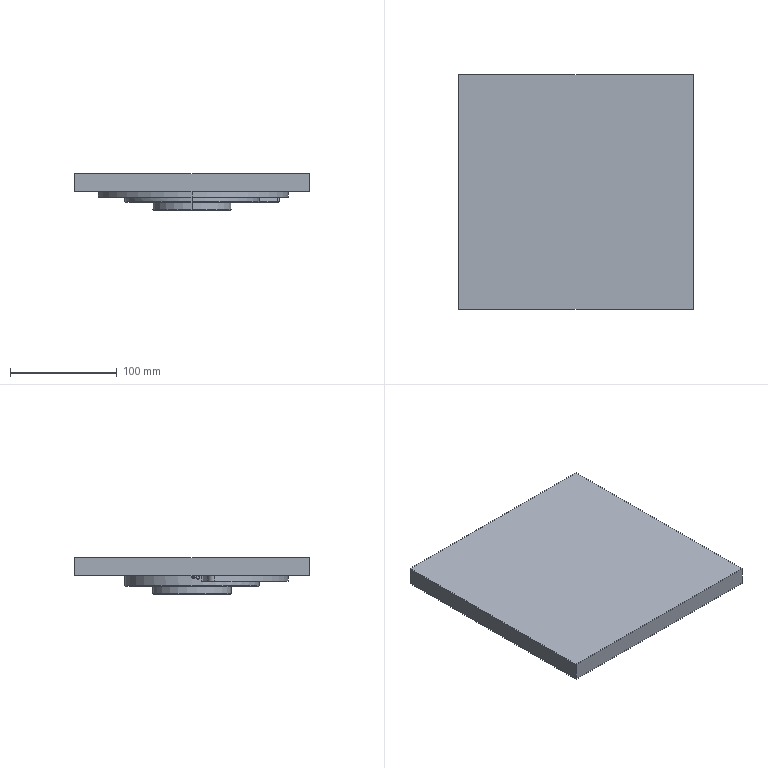Part | 2 solids | 200 faces | box 220 x 220 x 34.5 mm | volume 894057 mm3 | cylinder 99 | cone 50 | plane 32 | spline 11 | torus 4 | sphere 4 | commonest cylinder face diameters 3.5 x12 5 x12 10 x12 2.5 x10 4 x7 0.5 x6